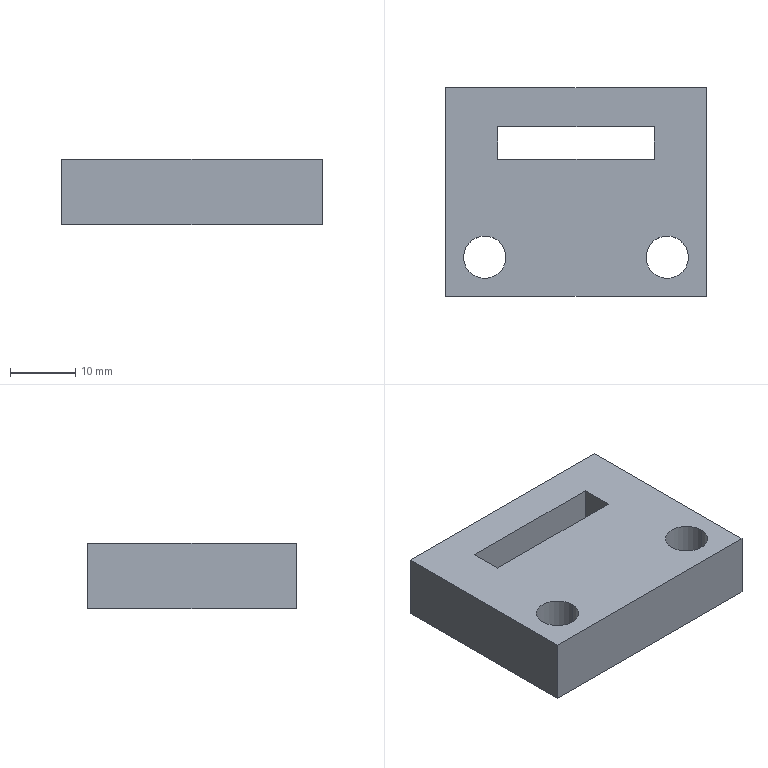Part | 1 solid | 14 faces | box 40 x 32 x 10 mm | volume 10615 mm3 | plane 10 | cylinder 4 | commonest cylinder face diameters 6.5 x4
STEP:
#1=CARTESIAN_POINT('',(10.75,0.,10.));
#2=VERTEX_POINT('',#1);
#3=CARTESIAN_POINT('',(17.25,0.,10.));
#4=VERTEX_POINT('',#3);
#5=CARTESIAN_POINT('',(14.,0.,10.));
#6=DIRECTION('',(0.,0.,1.));
#7=DIRECTION('',(1.,0.,0.));
#8=AXIS2_PLACEMENT_3D('',#5,#6,#7);
#9=CIRCLE('',#8,3.25);
#10=EDGE_CURVE('',#2,#4,#9,.T.);
#11=ORIENTED_EDGE('',*,*,#10,.T.);
#12=CARTESIAN_POINT('',(17.25,0.,0.));
#13=VERTEX_POINT('',#12);
#14=CARTESIAN_POINT('',(17.25,0.,10.));
#15=DIRECTION('',(0.,0.,-1.));
#16=VECTOR('',#15,1000.);
#17=LINE('',#14,#16);
#18=EDGE_CURVE('',#4,#13,#17,.T.);
#19=ORIENTED_EDGE('',*,*,#18,.T.);
#20=CARTESIAN_POINT('',(10.75,0.,0.));
#21=VERTEX_POINT('',#20);
#22=CARTESIAN_POINT('',(14.,0.,0.));
#23=DIRECTION('',(0.,0.,1.));
#24=DIRECTION('',(1.,0.,0.));
#25=AXIS2_PLACEMENT_3D('',#22,#23,#24);
#26=CIRCLE('',#25,3.25);
#27=EDGE_CURVE('',#21,#13,#26,.T.);
#28=ORIENTED_EDGE('',*,*,#27,.F.);
#29=CARTESIAN_POINT('',(10.75,0.,10.));
#30=DIRECTION('',(0.,0.,-1.));
#31=VECTOR('',#30,1000.);
#32=LINE('',#29,#31);
#33=EDGE_CURVE('',#2,#21,#32,.T.);
#34=ORIENTED_EDGE('',*,*,#33,.F.);
#35=EDGE_LOOP('',(#11,#19,#28,#34));
#36=FACE_OUTER_BOUND('',#35,.T.);
#37=CARTESIAN_POINT('',(14.,0.,10.));
#38=DIRECTION('',(0.,0.,-1.));
#39=DIRECTION('',(-1.,0.,0.));
#40=AXIS2_PLACEMENT_3D('',#37,#38,#39);
#41=CYLINDRICAL_SURFACE('',#40,3.25);
#42=ADVANCED_FACE('',(#36),#41,.F.);
#43=CARTESIAN_POINT('',(-17.25,0.,10.));
#44=VERTEX_POINT('',#43);
#45=CARTESIAN_POINT('',(-10.75,0.,10.));
#46=VERTEX_POINT('',#45);
#47=CARTESIAN_POINT('',(-14.,0.,10.));
#48=DIRECTION('',(0.,0.,1.));
#49=DIRECTION('',(1.,0.,0.));
#50=AXIS2_PLACEMENT_3D('',#47,#48,#49);
#51=CIRCLE('',#50,3.25);
#52=EDGE_CURVE('',#44,#46,#51,.T.);
#53=ORIENTED_EDGE('',*,*,#52,.T.);
#54=CARTESIAN_POINT('',(-10.75,0.,0.));
#55=VERTEX_POINT('',#54);
#56=CARTESIAN_POINT('',(-10.75,0.,10.));
#57=DIRECTION('',(0.,0.,-1.));
#58=VECTOR('',#57,1000.);
#59=LINE('',#56,#58);
#60=EDGE_CURVE('',#46,#55,#59,.T.);
#61=ORIENTED_EDGE('',*,*,#60,.T.);
#62=CARTESIAN_POINT('',(-17.25,0.,0.));
#63=VERTEX_POINT('',#62);
#64=CARTESIAN_POINT('',(-14.,0.,0.));
#65=DIRECTION('',(0.,0.,1.));
#66=DIRECTION('',(1.,0.,0.));
#67=AXIS2_PLACEMENT_3D('',#64,#65,#66);
#68=CIRCLE('',#67,3.25);
#69=EDGE_CURVE('',#63,#55,#68,.T.);
#70=ORIENTED_EDGE('',*,*,#69,.F.);
#71=CARTESIAN_POINT('',(-17.25,0.,10.));
#72=DIRECTION('',(0.,0.,-1.));
#73=VECTOR('',#72,1000.);
#74=LINE('',#71,#73);
#75=EDGE_CURVE('',#44,#63,#74,.T.);
#76=ORIENTED_EDGE('',*,*,#75,.F.);
#77=EDGE_LOOP('',(#53,#61,#70,#76));
#78=FACE_OUTER_BOUND('',#77,.T.);
#79=CARTESIAN_POINT('',(-14.,0.,10.));
#80=DIRECTION('',(0.,0.,-1.));
#81=DIRECTION('',(-1.,0.,0.));
#82=AXIS2_PLACEMENT_3D('',#79,#80,#81);
#83=CYLINDRICAL_SURFACE('',#82,3.25);
#84=ADVANCED_FACE('',(#78),#83,.F.);
#85=CARTESIAN_POINT('',(20.,-6.,10.));
#86=VERTEX_POINT('',#85);
#87=CARTESIAN_POINT('',(20.,26.,10.));
#88=VERTEX_POINT('',#87);
#89=CARTESIAN_POINT('',(20.,-6.,10.));
#90=DIRECTION('',(0.,1.,0.));
#91=VECTOR('',#90,1000.);
#92=LINE('',#89,#91);
#93=EDGE_CURVE('',#86,#88,#92,.T.);
#94=ORIENTED_EDGE('',*,*,#93,.T.);
#95=CARTESIAN_POINT('',(-20.,26.,10.));
#96=VERTEX_POINT('',#95);
#97=CARTESIAN_POINT('',(-20.,26.,10.));
#98=DIRECTION('',(-1.,0.,0.));
#99=VECTOR('',#98,1000.);
#100=LINE('',#97,#99);
#101=EDGE_CURVE('',#88,#96,#100,.T.);
#102=ORIENTED_EDGE('',*,*,#101,.T.);
#103=CARTESIAN_POINT('',(-20.,-6.,10.));
#104=VERTEX_POINT('',#103);
#105=CARTESIAN_POINT('',(-20.,-6.,10.));
#106=DIRECTION('',(0.,-1.,0.));
#107=VECTOR('',#106,1000.);
#108=LINE('',#105,#107);
#109=EDGE_CURVE('',#96,#104,#108,.T.);
#110=ORIENTED_EDGE('',*,*,#109,.T.);
#111=CARTESIAN_POINT('',(-20.,-6.,10.));
#112=DIRECTION('',(1.,0.,0.));
#113=VECTOR('',#112,1000.);
#114=LINE('',#111,#113);
#115=EDGE_CURVE('',#104,#86,#114,.T.);
#116=ORIENTED_EDGE('',*,*,#115,.T.);
#117=EDGE_LOOP('',(#94,#102,#110,#116));
#118=FACE_OUTER_BOUND('',#117,.T.);
#119=ORIENTED_EDGE('',*,*,#52,.F.);
#120=CARTESIAN_POINT('',(-14.,0.,10.));
#121=DIRECTION('',(0.,0.,1.));
#122=DIRECTION('',(1.,0.,0.));
#123=AXIS2_PLACEMENT_3D('',#120,#121,#122);
#124=CIRCLE('',#123,3.25);
#125=EDGE_CURVE('',#46,#44,#124,.T.);
#126=ORIENTED_EDGE('',*,*,#125,.F.);
#127=EDGE_LOOP('',(#119,#126));
#128=FACE_BOUND('',#127,.T.);
#129=ORIENTED_EDGE('',*,*,#10,.F.);
#130=CARTESIAN_POINT('',(14.,0.,10.));
#131=DIRECTION('',(0.,0.,1.));
#132=DIRECTION('',(1.,0.,0.));
#133=AXIS2_PLACEMENT_3D('',#130,#131,#132);
#134=CIRCLE('',#133,3.25);
#135=EDGE_CURVE('',#4,#2,#134,.T.);
#136=ORIENTED_EDGE('',*,*,#135,.F.);
#137=EDGE_LOOP('',(#129,#136));
#138=FACE_BOUND('',#137,.T.);
#139=CARTESIAN_POINT('',(-12.,15.,10.));
#140=VERTEX_POINT('',#139);
#141=CARTESIAN_POINT('',(12.,15.,10.));
#142=VERTEX_POINT('',#141);
#143=CARTESIAN_POINT('',(-12.,15.,10.));
#144=DIRECTION('',(1.,0.,0.));
#145=VECTOR('',#144,1000.);
#146=LINE('',#143,#145);
#147=EDGE_CURVE('',#140,#142,#146,.T.);
#148=ORIENTED_EDGE('',*,*,#147,.F.);
#149=CARTESIAN_POINT('',(-12.,20.,10.));
#150=VERTEX_POINT('',#149);
#151=CARTESIAN_POINT('',(-12.,20.,10.));
#152=DIRECTION('',(0.,-1.,0.));
#153=VECTOR('',#152,1000.);
#154=LINE('',#151,#153);
#155=EDGE_CURVE('',#150,#140,#154,.T.);
#156=ORIENTED_EDGE('',*,*,#155,.F.);
#157=CARTESIAN_POINT('',(12.,20.,10.));
#158=VERTEX_POINT('',#157);
#159=CARTESIAN_POINT('',(-12.,20.,10.));
#160=DIRECTION('',(-1.,0.,0.));
#161=VECTOR('',#160,1000.);
#162=LINE('',#159,#161);
#163=EDGE_CURVE('',#158,#150,#162,.T.);
#164=ORIENTED_EDGE('',*,*,#163,.F.);
#165=CARTESIAN_POINT('',(12.,20.,10.));
#166=DIRECTION('',(0.,1.,0.));
#167=VECTOR('',#166,1000.);
#168=LINE('',#165,#167);
#169=EDGE_CURVE('',#142,#158,#168,.T.);
#170=ORIENTED_EDGE('',*,*,#169,.F.);
#171=EDGE_LOOP('',(#148,#156,#164,#170));
#172=FACE_BOUND('',#171,.T.);
#173=CARTESIAN_POINT('',(0.,0.,10.));
#174=DIRECTION('',(0.,0.,-1.));
#175=DIRECTION('',(-1.,0.,0.));
#176=AXIS2_PLACEMENT_3D('',#173,#174,#175);
#177=PLANE('',#176);
#178=ADVANCED_FACE('',(#118,#128,#138,#172),#177,.F.);
#179=ORIENTED_EDGE('',*,*,#69,.T.);
#180=CARTESIAN_POINT('',(-14.,0.,0.));
#181=DIRECTION('',(0.,0.,1.));
#182=DIRECTION('',(1.,0.,0.));
#183=AXIS2_PLACEMENT_3D('',#180,#181,#182);
#184=CIRCLE('',#183,3.25);
#185=EDGE_CURVE('',#55,#63,#184,.T.);
#186=ORIENTED_EDGE('',*,*,#185,.T.);
#187=EDGE_LOOP('',(#179,#186));
#188=FACE_BOUND('',#187,.T.);
#189=CARTESIAN_POINT('',(20.,-6.,0.));
#190=VERTEX_POINT('',#189);
#191=CARTESIAN_POINT('',(20.,26.,0.));
#192=VERTEX_POINT('',#191);
#193=CARTESIAN_POINT('',(20.,-6.,0.));
#194=DIRECTION('',(0.,1.,0.));
#195=VECTOR('',#194,1000.);
#196=LINE('',#193,#195);
#197=EDGE_CURVE('',#190,#192,#196,.T.);
#198=ORIENTED_EDGE('',*,*,#197,.F.);
#199=CARTESIAN_POINT('',(-20.,-6.,0.));
#200=VERTEX_POINT('',#199);
#201=CARTESIAN_POINT('',(-20.,-6.,0.));
#202=DIRECTION('',(1.,0.,0.));
#203=VECTOR('',#202,1000.);
#204=LINE('',#201,#203);
#205=EDGE_CURVE('',#200,#190,#204,.T.);
#206=ORIENTED_EDGE('',*,*,#205,.F.);
#207=CARTESIAN_POINT('',(-20.,26.,0.));
#208=VERTEX_POINT('',#207);
#209=CARTESIAN_POINT('',(-20.,-6.,0.));
#210=DIRECTION('',(0.,-1.,0.));
#211=VECTOR('',#210,1000.);
#212=LINE('',#209,#211);
#213=EDGE_CURVE('',#208,#200,#212,.T.);
#214=ORIENTED_EDGE('',*,*,#213,.F.);
#215=CARTESIAN_POINT('',(-20.,26.,0.));
#216=DIRECTION('',(-1.,0.,0.));
#217=VECTOR('',#216,1000.);
#218=LINE('',#215,#217);
#219=EDGE_CURVE('',#192,#208,#218,.T.);
#220=ORIENTED_EDGE('',*,*,#219,.F.);
#221=EDGE_LOOP('',(#198,#206,#214,#220));
#222=FACE_OUTER_BOUND('',#221,.T.);
#223=ORIENTED_EDGE('',*,*,#27,.T.);
#224=CARTESIAN_POINT('',(14.,0.,0.));
#225=DIRECTION('',(0.,0.,1.));
#226=DIRECTION('',(1.,0.,0.));
#227=AXIS2_PLACEMENT_3D('',#224,#225,#226);
#228=CIRCLE('',#227,3.25);
#229=EDGE_CURVE('',#13,#21,#228,.T.);
#230=ORIENTED_EDGE('',*,*,#229,.T.);
#231=EDGE_LOOP('',(#223,#230));
#232=FACE_BOUND('',#231,.T.);
#233=CARTESIAN_POINT('',(-12.,12.321,0.));
#234=VERTEX_POINT('',#233);
#235=CARTESIAN_POINT('',(12.,12.321,0.));
#236=VERTEX_POINT('',#235);
#237=CARTESIAN_POINT('',(12.,12.321,0.));
#238=DIRECTION('',(1.,0.,0.));
#239=VECTOR('',#238,1000.);
#240=LINE('',#237,#239);
#241=EDGE_CURVE('',#234,#236,#240,.T.);
#242=ORIENTED_EDGE('',*,*,#241,.T.);
#243=CARTESIAN_POINT('',(12.,20.,0.));
#244=VERTEX_POINT('',#243);
#245=CARTESIAN_POINT('',(12.,20.,0.));
#246=DIRECTION('',(0.,1.,0.));
#247=VECTOR('',#246,1000.);
#248=LINE('',#245,#247);
#249=EDGE_CURVE('',#236,#244,#248,.T.);
#250=ORIENTED_EDGE('',*,*,#249,.T.);
#251=CARTESIAN_POINT('',(-12.,20.,0.));
#252=VERTEX_POINT('',#251);
#253=CARTESIAN_POINT('',(-12.,20.,0.));
#254=DIRECTION('',(-1.,0.,0.));
#255=VECTOR('',#254,1000.);
#256=LINE('',#253,#255);
#257=EDGE_CURVE('',#244,#252,#256,.T.);
#258=ORIENTED_EDGE('',*,*,#257,.T.);
#259=CARTESIAN_POINT('',(-12.,20.,0.));
#260=DIRECTION('',(0.,-1.,0.));
#261=VECTOR('',#260,1000.);
#262=LINE('',#259,#261);
#263=EDGE_CURVE('',#252,#234,#262,.T.);
#264=ORIENTED_EDGE('',*,*,#263,.T.);
#265=EDGE_LOOP('',(#242,#250,#258,#264));
#266=FACE_BOUND('',#265,.T.);
#267=CARTESIAN_POINT('',(0.,0.,0.));
#268=DIRECTION('',(0.,0.,-1.));
#269=DIRECTION('',(-1.,0.,0.));
#270=AXIS2_PLACEMENT_3D('',#267,#268,#269);
#271=PLANE('',#270);
#272=ADVANCED_FACE('',(#188,#222,#232,#266),#271,.T.);
#273=ORIENTED_EDGE('',*,*,#197,.T.);
#274=CARTESIAN_POINT('',(20.,26.,-44.721));
#275=DIRECTION('',(0.,0.,1.));
#276=VECTOR('',#275,1000.);
#277=LINE('',#274,#276);
#278=EDGE_CURVE('',#192,#88,#277,.T.);
#279=ORIENTED_EDGE('',*,*,#278,.T.);
#280=ORIENTED_EDGE('',*,*,#93,.F.);
#281=CARTESIAN_POINT('',(20.,-6.,10.));
#282=DIRECTION('',(0.,0.,-1.));
#283=VECTOR('',#282,1000.);
#284=LINE('',#281,#283);
#285=EDGE_CURVE('',#86,#190,#284,.T.);
#286=ORIENTED_EDGE('',*,*,#285,.T.);
#287=EDGE_LOOP('',(#273,#279,#280,#286));
#288=FACE_OUTER_BOUND('',#287,.T.);
#289=CARTESIAN_POINT('',(20.,-6.,10.));
#290=DIRECTION('',(-1.,0.,0.));
#291=DIRECTION('',(0.,0.,1.));
#292=AXIS2_PLACEMENT_3D('',#289,#290,#291);
#293=PLANE('',#292);
#294=ADVANCED_FACE('',(#288),#293,.F.);
#295=ORIENTED_EDGE('',*,*,#213,.T.);
#296=CARTESIAN_POINT('',(-20.,-6.,10.));
#297=DIRECTION('',(0.,0.,-1.));
#298=VECTOR('',#297,1000.);
#299=LINE('',#296,#298);
#300=EDGE_CURVE('',#104,#200,#299,.T.);
#301=ORIENTED_EDGE('',*,*,#300,.F.);
#302=ORIENTED_EDGE('',*,*,#109,.F.);
#303=CARTESIAN_POINT('',(-20.,26.,-44.721));
#304=DIRECTION('',(0.,0.,1.));
#305=VECTOR('',#304,1000.);
#306=LINE('',#303,#305);
#307=EDGE_CURVE('',#208,#96,#306,.T.);
#308=ORIENTED_EDGE('',*,*,#307,.F.);
#309=EDGE_LOOP('',(#295,#301,#302,#308));
#310=FACE_OUTER_BOUND('',#309,.T.);
#311=CARTESIAN_POINT('',(-20.,-6.,10.));
#312=DIRECTION('',(1.,0.,0.));
#313=DIRECTION('',(0.,0.,-1.));
#314=AXIS2_PLACEMENT_3D('',#311,#312,#313);
#315=PLANE('',#314);
#316=ADVANCED_FACE('',(#310),#315,.F.);
#317=ORIENTED_EDGE('',*,*,#205,.T.);
#318=ORIENTED_EDGE('',*,*,#285,.F.);
#319=ORIENTED_EDGE('',*,*,#115,.F.);
#320=ORIENTED_EDGE('',*,*,#300,.T.);
#321=EDGE_LOOP('',(#317,#318,#319,#320));
#322=FACE_OUTER_BOUND('',#321,.T.);
#323=CARTESIAN_POINT('',(-20.,-6.,10.));
#324=DIRECTION('',(0.,1.,0.));
#325=DIRECTION('',(0.,0.,1.));
#326=AXIS2_PLACEMENT_3D('',#323,#324,#325);
#327=PLANE('',#326);
#328=ADVANCED_FACE('',(#322),#327,.F.);
#329=ORIENTED_EDGE('',*,*,#60,.F.);
#330=ORIENTED_EDGE('',*,*,#125,.T.);
#331=ORIENTED_EDGE('',*,*,#75,.T.);
#332=ORIENTED_EDGE('',*,*,#185,.F.);
#333=EDGE_LOOP('',(#329,#330,#331,#332));
#334=FACE_OUTER_BOUND('',#333,.T.);
#335=CARTESIAN_POINT('',(-14.,0.,10.));
#336=DIRECTION('',(0.,0.,-1.));
#337=DIRECTION('',(-1.,0.,0.));
#338=AXIS2_PLACEMENT_3D('',#335,#336,#337);
#339=CYLINDRICAL_SURFACE('',#338,3.25);
#340=ADVANCED_FACE('',(#334),#339,.F.);
#341=ORIENTED_EDGE('',*,*,#18,.F.);
#342=ORIENTED_EDGE('',*,*,#135,.T.);
#343=ORIENTED_EDGE('',*,*,#33,.T.);
#344=ORIENTED_EDGE('',*,*,#229,.F.);
#345=EDGE_LOOP('',(#341,#342,#343,#344));
#346=FACE_OUTER_BOUND('',#345,.T.);
#347=CARTESIAN_POINT('',(14.,0.,10.));
#348=DIRECTION('',(0.,0.,-1.));
#349=DIRECTION('',(-1.,0.,0.));
#350=AXIS2_PLACEMENT_3D('',#347,#348,#349);
#351=CYLINDRICAL_SURFACE('',#350,3.25);
#352=ADVANCED_FACE('',(#346),#351,.F.);
#353=ORIENTED_EDGE('',*,*,#278,.F.);
#354=ORIENTED_EDGE('',*,*,#219,.T.);
#355=ORIENTED_EDGE('',*,*,#307,.T.);
#356=ORIENTED_EDGE('',*,*,#101,.F.);
#357=EDGE_LOOP('',(#353,#354,#355,#356));
#358=FACE_OUTER_BOUND('',#357,.T.);
#359=CARTESIAN_POINT('',(-20.,26.,-44.721));
#360=DIRECTION('',(0.,1.,0.));
#361=DIRECTION('',(0.,0.,1.));
#362=AXIS2_PLACEMENT_3D('',#359,#360,#361);
#363=PLANE('',#362);
#364=ADVANCED_FACE('',(#358),#363,.T.);
#365=ORIENTED_EDGE('',*,*,#263,.F.);
#366=CARTESIAN_POINT('',(-12.,20.,-44.721));
#367=DIRECTION('',(0.,0.,1.));
#368=VECTOR('',#367,1000.);
#369=LINE('',#366,#368);
#370=EDGE_CURVE('',#252,#150,#369,.T.);
#371=ORIENTED_EDGE('',*,*,#370,.T.);
#372=ORIENTED_EDGE('',*,*,#155,.T.);
#373=CARTESIAN_POINT('',(-12.,1.655,-39.806));
#374=DIRECTION('',(0.,-0.2588,-0.9659));
#375=VECTOR('',#374,1000.);
#376=LINE('',#373,#375);
#377=EDGE_CURVE('',#140,#234,#376,.T.);
#378=ORIENTED_EDGE('',*,*,#377,.T.);
#379=EDGE_LOOP('',(#365,#371,#372,#378));
#380=FACE_OUTER_BOUND('',#379,.T.);
#381=CARTESIAN_POINT('',(-12.,20.,-44.721));
#382=DIRECTION('',(-1.,0.,0.));
#383=DIRECTION('',(0.,-1.,0.));
#384=AXIS2_PLACEMENT_3D('',#381,#382,#383);
#385=PLANE('',#384);
#386=ADVANCED_FACE('',(#380),#385,.F.);
#387=ORIENTED_EDGE('',*,*,#257,.F.);
#388=CARTESIAN_POINT('',(12.,20.,-44.721));
#389=DIRECTION('',(0.,0.,1.));
#390=VECTOR('',#389,1000.);
#391=LINE('',#388,#390);
#392=EDGE_CURVE('',#244,#158,#391,.T.);
#393=ORIENTED_EDGE('',*,*,#392,.T.);
#394=ORIENTED_EDGE('',*,*,#163,.T.);
#395=ORIENTED_EDGE('',*,*,#370,.F.);
#396=EDGE_LOOP('',(#387,#393,#394,#395));
#397=FACE_OUTER_BOUND('',#396,.T.);
#398=CARTESIAN_POINT('',(-12.,20.,-44.721));
#399=DIRECTION('',(0.,1.,0.));
#400=DIRECTION('',(0.,0.,1.));
#401=AXIS2_PLACEMENT_3D('',#398,#399,#400);
#402=PLANE('',#401);
#403=ADVANCED_FACE('',(#397),#402,.F.);
#404=ORIENTED_EDGE('',*,*,#249,.F.);
#405=CARTESIAN_POINT('',(12.,1.655,-39.806));
#406=DIRECTION('',(0.,0.2588,0.9659));
#407=VECTOR('',#406,1000.);
#408=LINE('',#405,#407);
#409=EDGE_CURVE('',#236,#142,#408,.T.);
#410=ORIENTED_EDGE('',*,*,#409,.T.);
#411=ORIENTED_EDGE('',*,*,#169,.T.);
#412=ORIENTED_EDGE('',*,*,#392,.F.);
#413=EDGE_LOOP('',(#404,#410,#411,#412));
#414=FACE_OUTER_BOUND('',#413,.T.);
#415=CARTESIAN_POINT('',(12.,20.,-44.721));
#416=DIRECTION('',(1.,0.,0.));
#417=DIRECTION('',(0.,1.,0.));
#418=AXIS2_PLACEMENT_3D('',#415,#416,#417);
#419=PLANE('',#418);
#420=ADVANCED_FACE('',(#414),#419,.F.);
#421=ORIENTED_EDGE('',*,*,#377,.F.);
#422=ORIENTED_EDGE('',*,*,#147,.T.);
#423=ORIENTED_EDGE('',*,*,#409,.F.);
#424=ORIENTED_EDGE('',*,*,#241,.F.);
#425=EDGE_LOOP('',(#421,#422,#423,#424));
#426=FACE_OUTER_BOUND('',#425,.T.);
#427=CARTESIAN_POINT('',(0.,12.321,0.));
#428=DIRECTION('',(0.,0.9659,-0.2588));
#429=DIRECTION('',(-1.,0.,0.));
#430=AXIS2_PLACEMENT_3D('',#427,#428,#429);
#431=PLANE('',#430);
#432=ADVANCED_FACE('',(#426),#431,.T.);
#433=CLOSED_SHELL('',(#42,#84,#178,#272,#294,#316,#328,#340,#352,#364,#386,#403,#420,#432));
#434=MANIFOLD_SOLID_BREP('',#433);
#435=CARTESIAN_POINT('',(0.,0.,0.));
#436=DIRECTION('',(0.,0.,1.));
#437=DIRECTION('',(1.,0.,0.));
#438=AXIS2_PLACEMENT_3D('',#435,#436,#437);
#439=(LENGTH_UNIT()NAMED_UNIT(*)SI_UNIT(.MILLI.,.METRE.));
#440=UNCERTAINTY_MEASURE_WITH_UNIT(LENGTH_MEASURE(0.00001),#439,'','');
#441=(NAMED_UNIT(*)PLANE_ANGLE_UNIT()SI_UNIT($,.RADIAN.));
#442=(NAMED_UNIT(*)SI_UNIT($,.STERADIAN.)SOLID_ANGLE_UNIT());
#443=(GEOMETRIC_REPRESENTATION_CONTEXT(3)GLOBAL_UNCERTAINTY_ASSIGNED_CONTEXT((#440))GLOBAL_UNIT_ASSIGNED_CONTEXT((#439,#441,#442))REPRESENTATION_CONTEXT('',''));
#444=ADVANCED_BREP_SHAPE_REPRESENTATION('',(#434,#438),#443);